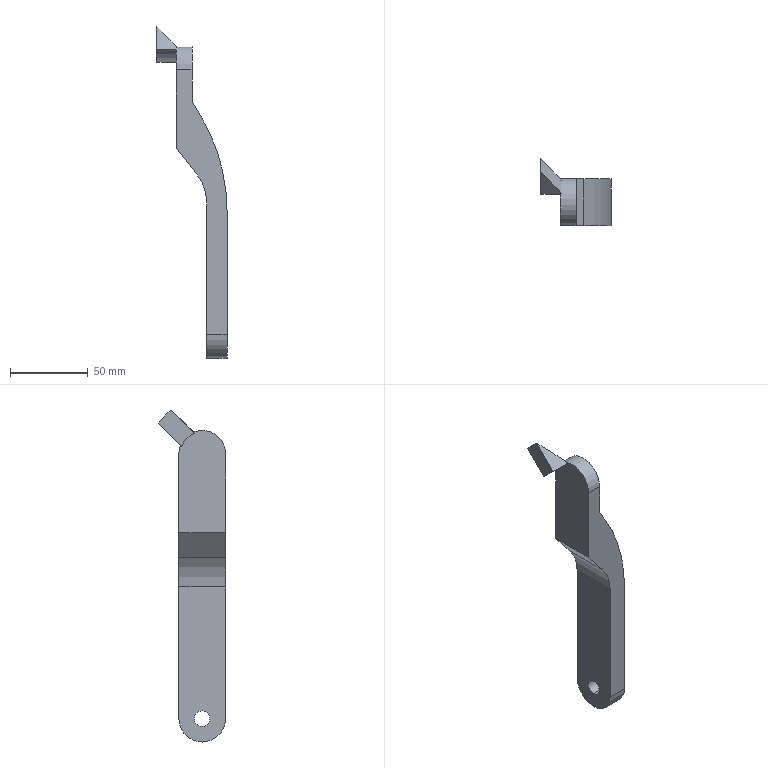Part | STEP file | Pedal RHS | 2 solids | 20 faces | box 45 x 43.067 x 213.067 mm | volume 82900 mm3 | plane 11 | cylinder 8 | cone 1 | commonest cylinder face diameters 30 x3 10 x2 28.237 x1 60 x1 240 x1